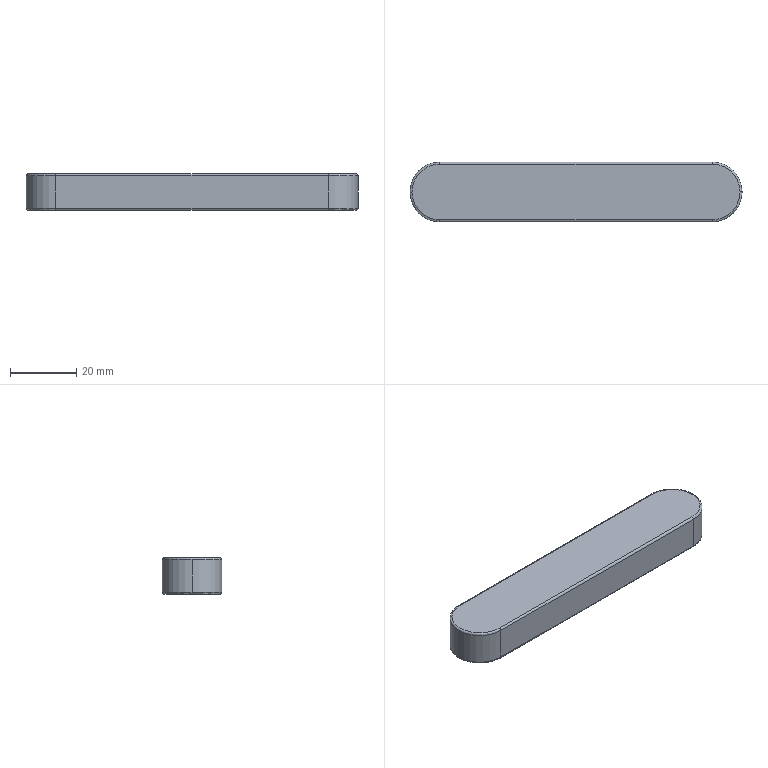Part | STEP file | 1 solid | 17 faces | box 100 x 18 x 11 mm | volume 19001 mm3 | cylinder 7 | spline 6 | plane 4 | commonest cylinder face diameters 1.2 x4 18 x3